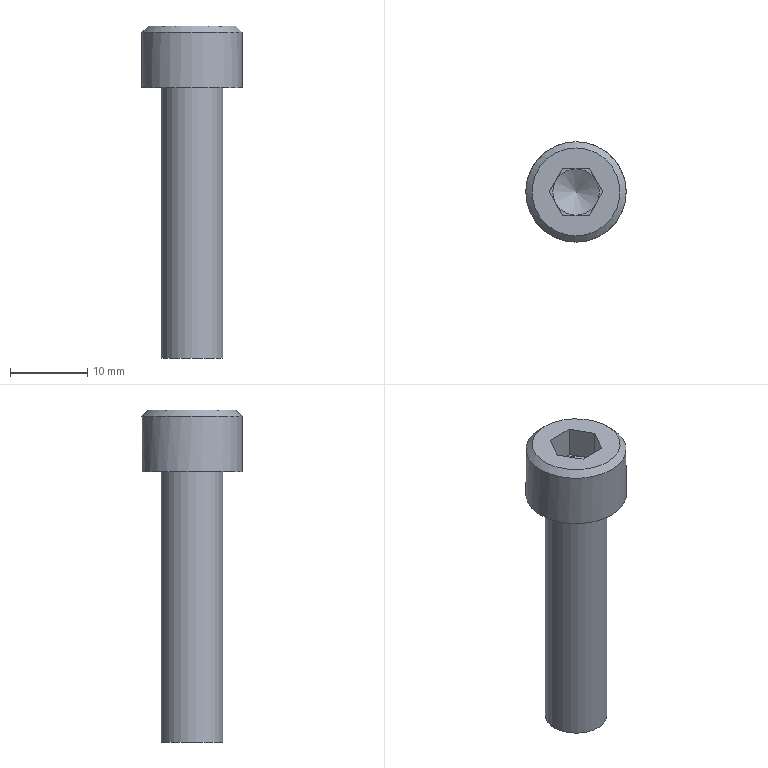Part | NX | features 5003_330_CB8-35 2 | 1 solid | 19 faces | box 13 x 13 x 43 mm | volume 2667 mm3 | plane 15 | cylinder 2 | cone 2 | commonest cylinder face diameters 8 x1 13 x1
STEP:
#1=CARTESIAN_POINT('',(-1.475,-243.8,-208.5));
#2=VERTEX_POINT('',#1);
#3=CARTESIAN_POINT('',(-1.475,-249.5,-208.5));
#4=DIRECTION('',(0.,0.,-1.));
#5=DIRECTION('',(0.,1.,0.));
#6=AXIS2_PLACEMENT_3D('',#3,#4,#5);
#7=CIRCLE('',#6,5.7);
#8=EDGE_CURVE('',#2,#2,#7,.F.);
#9=ORIENTED_EDGE('',*,*,#8,.T.);
#10=EDGE_LOOP('',(#9));
#11=FACE_BOUND('',#10,.T.);
#12=CARTESIAN_POINT('',(-4.939,-249.5,-208.5));
#13=VERTEX_POINT('',#12);
#14=CARTESIAN_POINT('',(-3.207,-252.5,-208.5));
#15=VERTEX_POINT('',#14);
#16=CARTESIAN_POINT('',(-4.939,-249.5,-208.5));
#17=DIRECTION('',(0.5,-0.866,0.));
#18=VECTOR('',#17,1000.);
#19=LINE('',#16,#18);
#20=EDGE_CURVE('',#13,#15,#19,.T.);
#21=ORIENTED_EDGE('',*,*,#20,.F.);
#22=CARTESIAN_POINT('',(-3.207,-246.5,-208.5));
#23=VERTEX_POINT('',#22);
#24=CARTESIAN_POINT('',(-3.207,-246.5,-208.5));
#25=DIRECTION('',(-0.5,-0.866,0.));
#26=VECTOR('',#25,1000.);
#27=LINE('',#24,#26);
#28=EDGE_CURVE('',#23,#13,#27,.T.);
#29=ORIENTED_EDGE('',*,*,#28,.F.);
#30=CARTESIAN_POINT('',(0.2571,-246.5,-208.5));
#31=VERTEX_POINT('',#30);
#32=CARTESIAN_POINT('',(0.2571,-246.5,-208.5));
#33=DIRECTION('',(-1.,0.,0.));
#34=VECTOR('',#33,1000.);
#35=LINE('',#32,#34);
#36=EDGE_CURVE('',#31,#23,#35,.T.);
#37=ORIENTED_EDGE('',*,*,#36,.F.);
#38=CARTESIAN_POINT('',(1.989,-249.5,-208.5));
#39=VERTEX_POINT('',#38);
#40=CARTESIAN_POINT('',(1.989,-249.5,-208.5));
#41=DIRECTION('',(-0.5,0.866,0.));
#42=VECTOR('',#41,1000.);
#43=LINE('',#40,#42);
#44=EDGE_CURVE('',#39,#31,#43,.T.);
#45=ORIENTED_EDGE('',*,*,#44,.F.);
#46=CARTESIAN_POINT('',(0.2571,-252.5,-208.5));
#47=VERTEX_POINT('',#46);
#48=CARTESIAN_POINT('',(0.2571,-252.5,-208.5));
#49=DIRECTION('',(0.5,0.866,0.));
#50=VECTOR('',#49,1000.);
#51=LINE('',#48,#50);
#52=EDGE_CURVE('',#47,#39,#51,.T.);
#53=ORIENTED_EDGE('',*,*,#52,.F.);
#54=CARTESIAN_POINT('',(-3.207,-252.5,-208.5));
#55=DIRECTION('',(1.,0.,0.));
#56=VECTOR('',#55,1000.);
#57=LINE('',#54,#56);
#58=EDGE_CURVE('',#15,#47,#57,.T.);
#59=ORIENTED_EDGE('',*,*,#58,.F.);
#60=EDGE_LOOP('',(#21,#29,#37,#45,#53,#59));
#61=FACE_BOUND('',#60,.T.);
#62=CARTESIAN_POINT('',(5.025,-249.5,-208.5));
#63=DIRECTION('',(0.,0.,-1.));
#64=DIRECTION('',(0.,1.,0.));
#65=AXIS2_PLACEMENT_3D('',#62,#63,#64);
#66=PLANE('',#65);
#67=ADVANCED_FACE('',(#11,#61),#66,.F.);
#68=CARTESIAN_POINT('',(-1.475,-253.5,-251.5));
#69=VERTEX_POINT('',#68);
#70=CARTESIAN_POINT('',(-1.475,-249.5,-251.5));
#71=DIRECTION('',(0.,0.,1.));
#72=DIRECTION('',(0.,-1.,0.));
#73=AXIS2_PLACEMENT_3D('',#70,#71,#72);
#74=CIRCLE('',#73,4.);
#75=EDGE_CURVE('',#69,#69,#74,.T.);
#76=ORIENTED_EDGE('',*,*,#75,.F.);
#77=EDGE_LOOP('',(#76));
#78=FACE_BOUND('',#77,.T.);
#79=CARTESIAN_POINT('',(-1.475,-249.5,-251.5));
#80=DIRECTION('',(0.,0.,1.));
#81=DIRECTION('',(0.,-1.,0.));
#82=AXIS2_PLACEMENT_3D('',#79,#80,#81);
#83=PLANE('',#82);
#84=ADVANCED_FACE('',(#78),#83,.F.);
#85=CARTESIAN_POINT('',(-1.475,-253.5,-216.5));
#86=VERTEX_POINT('',#85);
#87=CARTESIAN_POINT('',(-1.475,-249.5,-216.5));
#88=DIRECTION('',(0.,0.,1.));
#89=DIRECTION('',(0.,-1.,0.));
#90=AXIS2_PLACEMENT_3D('',#87,#88,#89);
#91=CIRCLE('',#90,4.);
#92=EDGE_CURVE('',#86,#86,#91,.T.);
#93=ORIENTED_EDGE('',*,*,#92,.F.);
#94=EDGE_LOOP('',(#93));
#95=FACE_BOUND('',#94,.T.);
#96=ORIENTED_EDGE('',*,*,#75,.T.);
#97=EDGE_LOOP('',(#96));
#98=FACE_BOUND('',#97,.T.);
#99=CARTESIAN_POINT('',(-1.475,-249.5,-208.5));
#100=DIRECTION('',(0.,0.,1.));
#101=DIRECTION('',(0.,-1.,0.));
#102=AXIS2_PLACEMENT_3D('',#99,#100,#101);
#103=CYLINDRICAL_SURFACE('',#102,4.);
#104=ADVANCED_FACE('',(#95,#98),#103,.T.);
#105=CARTESIAN_POINT('',(-1.475,-256.,-216.5));
#106=VERTEX_POINT('',#105);
#107=CARTESIAN_POINT('',(-1.475,-249.5,-216.5));
#108=DIRECTION('',(0.,0.,1.));
#109=DIRECTION('',(0.,-1.,0.));
#110=AXIS2_PLACEMENT_3D('',#107,#108,#109);
#111=CIRCLE('',#110,6.5);
#112=EDGE_CURVE('',#106,#106,#111,.T.);
#113=ORIENTED_EDGE('',*,*,#112,.F.);
#114=EDGE_LOOP('',(#113));
#115=FACE_BOUND('',#114,.T.);
#116=ORIENTED_EDGE('',*,*,#92,.T.);
#117=EDGE_LOOP('',(#116));
#118=FACE_BOUND('',#117,.T.);
#119=CARTESIAN_POINT('',(2.525,-249.5,-216.5));
#120=DIRECTION('',(0.,0.,1.));
#121=DIRECTION('',(0.,-1.,0.));
#122=AXIS2_PLACEMENT_3D('',#119,#120,#121);
#123=PLANE('',#122);
#124=ADVANCED_FACE('',(#115,#118),#123,.F.);
#125=CARTESIAN_POINT('',(-1.475,-243.,-209.3));
#126=VERTEX_POINT('',#125);
#127=CARTESIAN_POINT('',(-1.475,-249.5,-209.3));
#128=DIRECTION('',(0.,0.,-1.));
#129=DIRECTION('',(0.,1.,0.));
#130=AXIS2_PLACEMENT_3D('',#127,#128,#129);
#131=CIRCLE('',#130,6.5);
#132=EDGE_CURVE('',#126,#126,#131,.T.);
#133=ORIENTED_EDGE('',*,*,#132,.T.);
#134=EDGE_LOOP('',(#133));
#135=FACE_BOUND('',#134,.T.);
#136=ORIENTED_EDGE('',*,*,#112,.T.);
#137=EDGE_LOOP('',(#136));
#138=FACE_BOUND('',#137,.T.);
#139=CARTESIAN_POINT('',(-1.475,-249.5,-208.5));
#140=DIRECTION('',(0.,0.,1.));
#141=DIRECTION('',(0.,-1.,0.));
#142=AXIS2_PLACEMENT_3D('',#139,#140,#141);
#143=CYLINDRICAL_SURFACE('',#142,6.5);
#144=ADVANCED_FACE('',(#135,#138),#143,.T.);
#145=ORIENTED_EDGE('',*,*,#132,.F.);
#146=EDGE_LOOP('',(#145));
#147=FACE_BOUND('',#146,.T.);
#148=ORIENTED_EDGE('',*,*,#8,.F.);
#149=EDGE_LOOP('',(#148));
#150=FACE_BOUND('',#149,.T.);
#151=CARTESIAN_POINT('',(-1.475,-249.5,-208.5));
#152=DIRECTION('',(0.,0.,-1.));
#153=DIRECTION('',(0.,1.,0.));
#154=AXIS2_PLACEMENT_3D('',#151,#152,#153);
#155=CONICAL_SURFACE('',#154,5.7,0.7854);
#156=ADVANCED_FACE('',(#147,#150),#155,.T.);
#157=CARTESIAN_POINT('',(-3.207,-246.5,-212.5));
#158=VERTEX_POINT('',#157);
#159=CARTESIAN_POINT('',(-4.073,-248.,-212.5));
#160=VERTEX_POINT('',#159);
#161=CARTESIAN_POINT('',(-3.207,-246.5,-212.5));
#162=DIRECTION('',(-0.5,-0.866,0.));
#163=VECTOR('',#162,1000.);
#164=LINE('',#161,#163);
#165=EDGE_CURVE('',#158,#160,#164,.T.);
#166=ORIENTED_EDGE('',*,*,#165,.F.);
#167=CARTESIAN_POINT('',(-3.207,-246.5,-212.5));
#168=DIRECTION('',(0.,0.,1.));
#169=VECTOR('',#168,1000.);
#170=LINE('',#167,#169);
#171=EDGE_CURVE('',#158,#23,#170,.T.);
#172=ORIENTED_EDGE('',*,*,#171,.T.);
#173=ORIENTED_EDGE('',*,*,#28,.T.);
#174=CARTESIAN_POINT('',(-4.939,-249.5,-212.5));
#175=VERTEX_POINT('',#174);
#176=CARTESIAN_POINT('',(-4.939,-249.5,-212.5));
#177=DIRECTION('',(0.,0.,1.));
#178=VECTOR('',#177,1000.);
#179=LINE('',#176,#178);
#180=EDGE_CURVE('',#175,#13,#179,.T.);
#181=ORIENTED_EDGE('',*,*,#180,.F.);
#182=CARTESIAN_POINT('',(-3.207,-246.5,-212.5));
#183=DIRECTION('',(-0.5,-0.866,0.));
#184=VECTOR('',#183,1000.);
#185=LINE('',#182,#184);
#186=EDGE_CURVE('',#160,#175,#185,.T.);
#187=ORIENTED_EDGE('',*,*,#186,.F.);
#188=EDGE_LOOP('',(#166,#172,#173,#181,#187));
#189=FACE_BOUND('',#188,.T.);
#190=CARTESIAN_POINT('',(-3.207,-246.5,-212.5));
#191=DIRECTION('',(-0.866,0.5,0.));
#192=DIRECTION('',(0.5,0.866,0.));
#193=AXIS2_PLACEMENT_3D('',#190,#191,#192);
#194=PLANE('',#193);
#195=ADVANCED_FACE('',(#189),#194,.F.);
#196=CARTESIAN_POINT('',(0.2571,-246.5,-212.5));
#197=VERTEX_POINT('',#196);
#198=CARTESIAN_POINT('',(-1.475,-246.5,-212.5));
#199=VERTEX_POINT('',#198);
#200=CARTESIAN_POINT('',(0.2571,-246.5,-212.5));
#201=DIRECTION('',(-1.,0.,0.));
#202=VECTOR('',#201,1000.);
#203=LINE('',#200,#202);
#204=EDGE_CURVE('',#197,#199,#203,.T.);
#205=ORIENTED_EDGE('',*,*,#204,.F.);
#206=CARTESIAN_POINT('',(0.2571,-246.5,-212.5));
#207=DIRECTION('',(0.,0.,1.));
#208=VECTOR('',#207,1000.);
#209=LINE('',#206,#208);
#210=EDGE_CURVE('',#197,#31,#209,.T.);
#211=ORIENTED_EDGE('',*,*,#210,.T.);
#212=ORIENTED_EDGE('',*,*,#36,.T.);
#213=ORIENTED_EDGE('',*,*,#171,.F.);
#214=CARTESIAN_POINT('',(0.2571,-246.5,-212.5));
#215=DIRECTION('',(-1.,0.,0.));
#216=VECTOR('',#215,1000.);
#217=LINE('',#214,#216);
#218=EDGE_CURVE('',#199,#158,#217,.T.);
#219=ORIENTED_EDGE('',*,*,#218,.F.);
#220=EDGE_LOOP('',(#205,#211,#212,#213,#219));
#221=FACE_BOUND('',#220,.T.);
#222=CARTESIAN_POINT('',(0.2571,-246.5,-212.5));
#223=DIRECTION('',(0.,1.,0.));
#224=DIRECTION('',(0.,0.,1.));
#225=AXIS2_PLACEMENT_3D('',#222,#223,#224);
#226=PLANE('',#225);
#227=ADVANCED_FACE('',(#221),#226,.F.);
#228=CARTESIAN_POINT('',(1.989,-249.5,-212.5));
#229=VERTEX_POINT('',#228);
#230=CARTESIAN_POINT('',(1.123,-248.,-212.5));
#231=VERTEX_POINT('',#230);
#232=CARTESIAN_POINT('',(1.989,-249.5,-212.5));
#233=DIRECTION('',(-0.5,0.866,0.));
#234=VECTOR('',#233,1000.);
#235=LINE('',#232,#234);
#236=EDGE_CURVE('',#229,#231,#235,.T.);
#237=ORIENTED_EDGE('',*,*,#236,.F.);
#238=CARTESIAN_POINT('',(1.989,-249.5,-212.5));
#239=DIRECTION('',(0.,0.,1.));
#240=VECTOR('',#239,1000.);
#241=LINE('',#238,#240);
#242=EDGE_CURVE('',#229,#39,#241,.T.);
#243=ORIENTED_EDGE('',*,*,#242,.T.);
#244=ORIENTED_EDGE('',*,*,#44,.T.);
#245=ORIENTED_EDGE('',*,*,#210,.F.);
#246=CARTESIAN_POINT('',(1.989,-249.5,-212.5));
#247=DIRECTION('',(-0.5,0.866,0.));
#248=VECTOR('',#247,1000.);
#249=LINE('',#246,#248);
#250=EDGE_CURVE('',#231,#197,#249,.T.);
#251=ORIENTED_EDGE('',*,*,#250,.F.);
#252=EDGE_LOOP('',(#237,#243,#244,#245,#251));
#253=FACE_BOUND('',#252,.T.);
#254=CARTESIAN_POINT('',(1.989,-249.5,-212.5));
#255=DIRECTION('',(0.866,0.5,0.));
#256=DIRECTION('',(0.5,-0.866,0.));
#257=AXIS2_PLACEMENT_3D('',#254,#255,#256);
#258=PLANE('',#257);
#259=ADVANCED_FACE('',(#253),#258,.F.);
#260=CARTESIAN_POINT('',(0.2571,-252.5,-212.5));
#261=VERTEX_POINT('',#260);
#262=CARTESIAN_POINT('',(1.123,-251.,-212.5));
#263=VERTEX_POINT('',#262);
#264=CARTESIAN_POINT('',(0.2571,-252.5,-212.5));
#265=DIRECTION('',(0.5,0.866,0.));
#266=VECTOR('',#265,1000.);
#267=LINE('',#264,#266);
#268=EDGE_CURVE('',#261,#263,#267,.T.);
#269=ORIENTED_EDGE('',*,*,#268,.F.);
#270=CARTESIAN_POINT('',(0.2571,-252.5,-212.5));
#271=DIRECTION('',(0.,0.,1.));
#272=VECTOR('',#271,1000.);
#273=LINE('',#270,#272);
#274=EDGE_CURVE('',#261,#47,#273,.T.);
#275=ORIENTED_EDGE('',*,*,#274,.T.);
#276=ORIENTED_EDGE('',*,*,#52,.T.);
#277=ORIENTED_EDGE('',*,*,#242,.F.);
#278=CARTESIAN_POINT('',(0.2571,-252.5,-212.5));
#279=DIRECTION('',(0.5,0.866,0.));
#280=VECTOR('',#279,1000.);
#281=LINE('',#278,#280);
#282=EDGE_CURVE('',#263,#229,#281,.T.);
#283=ORIENTED_EDGE('',*,*,#282,.F.);
#284=EDGE_LOOP('',(#269,#275,#276,#277,#283));
#285=FACE_BOUND('',#284,.T.);
#286=CARTESIAN_POINT('',(0.2571,-252.5,-212.5));
#287=DIRECTION('',(0.866,-0.5,0.));
#288=DIRECTION('',(-0.5,-0.866,0.));
#289=AXIS2_PLACEMENT_3D('',#286,#287,#288);
#290=PLANE('',#289);
#291=ADVANCED_FACE('',(#285),#290,.F.);
#292=CARTESIAN_POINT('',(-3.207,-252.5,-212.5));
#293=VERTEX_POINT('',#292);
#294=CARTESIAN_POINT('',(-1.475,-252.5,-212.5));
#295=VERTEX_POINT('',#294);
#296=CARTESIAN_POINT('',(-3.207,-252.5,-212.5));
#297=DIRECTION('',(1.,0.,0.));
#298=VECTOR('',#297,1000.);
#299=LINE('',#296,#298);
#300=EDGE_CURVE('',#293,#295,#299,.T.);
#301=ORIENTED_EDGE('',*,*,#300,.F.);
#302=CARTESIAN_POINT('',(-3.207,-252.5,-212.5));
#303=DIRECTION('',(0.,0.,1.));
#304=VECTOR('',#303,1000.);
#305=LINE('',#302,#304);
#306=EDGE_CURVE('',#293,#15,#305,.T.);
#307=ORIENTED_EDGE('',*,*,#306,.T.);
#308=ORIENTED_EDGE('',*,*,#58,.T.);
#309=ORIENTED_EDGE('',*,*,#274,.F.);
#310=CARTESIAN_POINT('',(-3.207,-252.5,-212.5));
#311=DIRECTION('',(1.,0.,0.));
#312=VECTOR('',#311,1000.);
#313=LINE('',#310,#312);
#314=EDGE_CURVE('',#295,#261,#313,.T.);
#315=ORIENTED_EDGE('',*,*,#314,.F.);
#316=EDGE_LOOP('',(#301,#307,#308,#309,#315));
#317=FACE_BOUND('',#316,.T.);
#318=CARTESIAN_POINT('',(-3.207,-252.5,-212.5));
#319=DIRECTION('',(0.,-1.,0.));
#320=DIRECTION('',(-1.,0.,0.));
#321=AXIS2_PLACEMENT_3D('',#318,#319,#320);
#322=PLANE('',#321);
#323=ADVANCED_FACE('',(#317),#322,.F.);
#324=CARTESIAN_POINT('',(-4.073,-251.,-212.5));
#325=VERTEX_POINT('',#324);
#326=CARTESIAN_POINT('',(-4.939,-249.5,-212.5));
#327=DIRECTION('',(0.5,-0.866,0.));
#328=VECTOR('',#327,1000.);
#329=LINE('',#326,#328);
#330=EDGE_CURVE('',#175,#325,#329,.T.);
#331=ORIENTED_EDGE('',*,*,#330,.F.);
#332=ORIENTED_EDGE('',*,*,#180,.T.);
#333=ORIENTED_EDGE('',*,*,#20,.T.);
#334=ORIENTED_EDGE('',*,*,#306,.F.);
#335=CARTESIAN_POINT('',(-4.939,-249.5,-212.5));
#336=DIRECTION('',(0.5,-0.866,0.));
#337=VECTOR('',#336,1000.);
#338=LINE('',#335,#337);
#339=EDGE_CURVE('',#325,#293,#338,.T.);
#340=ORIENTED_EDGE('',*,*,#339,.F.);
#341=EDGE_LOOP('',(#331,#332,#333,#334,#340));
#342=FACE_BOUND('',#341,.T.);
#343=CARTESIAN_POINT('',(-4.939,-249.5,-212.5));
#344=DIRECTION('',(-0.866,-0.5,0.));
#345=DIRECTION('',(-0.5,0.866,0.));
#346=AXIS2_PLACEMENT_3D('',#343,#344,#345);
#347=PLANE('',#346);
#348=ADVANCED_FACE('',(#342),#347,.F.);
#349=ORIENTED_EDGE('',*,*,#314,.T.);
#350=ORIENTED_EDGE('',*,*,#268,.T.);
#351=CARTESIAN_POINT('',(-1.475,-249.5,-212.5));
#352=DIRECTION('',(0.,0.,1.));
#353=DIRECTION('',(-1.,0.,0.));
#354=AXIS2_PLACEMENT_3D('',#351,#352,#353);
#355=CIRCLE('',#354,3.);
#356=EDGE_CURVE('',#295,#263,#355,.T.);
#357=ORIENTED_EDGE('',*,*,#356,.F.);
#358=EDGE_LOOP('',(#349,#350,#357));
#359=FACE_BOUND('',#358,.T.);
#360=CARTESIAN_POINT('',(-1.475,-249.5,-212.5));
#361=DIRECTION('',(0.,0.,1.));
#362=DIRECTION('',(0.,-1.,0.));
#363=AXIS2_PLACEMENT_3D('',#360,#361,#362);
#364=PLANE('',#363);
#365=ADVANCED_FACE('',(#359),#364,.T.);
#366=ORIENTED_EDGE('',*,*,#282,.T.);
#367=ORIENTED_EDGE('',*,*,#236,.T.);
#368=CARTESIAN_POINT('',(-1.475,-249.5,-212.5));
#369=DIRECTION('',(0.,0.,1.));
#370=DIRECTION('',(-1.,0.,0.));
#371=AXIS2_PLACEMENT_3D('',#368,#369,#370);
#372=CIRCLE('',#371,3.);
#373=EDGE_CURVE('',#263,#231,#372,.T.);
#374=ORIENTED_EDGE('',*,*,#373,.F.);
#375=EDGE_LOOP('',(#366,#367,#374));
#376=FACE_BOUND('',#375,.T.);
#377=CARTESIAN_POINT('',(-1.475,-249.5,-212.5));
#378=DIRECTION('',(0.,0.,1.));
#379=DIRECTION('',(0.,-1.,0.));
#380=AXIS2_PLACEMENT_3D('',#377,#378,#379);
#381=PLANE('',#380);
#382=ADVANCED_FACE('',(#376),#381,.T.);
#383=ORIENTED_EDGE('',*,*,#250,.T.);
#384=ORIENTED_EDGE('',*,*,#204,.T.);
#385=CARTESIAN_POINT('',(-1.475,-249.5,-212.5));
#386=DIRECTION('',(0.,0.,1.));
#387=DIRECTION('',(-1.,0.,0.));
#388=AXIS2_PLACEMENT_3D('',#385,#386,#387);
#389=CIRCLE('',#388,3.);
#390=EDGE_CURVE('',#231,#199,#389,.T.);
#391=ORIENTED_EDGE('',*,*,#390,.F.);
#392=EDGE_LOOP('',(#383,#384,#391));
#393=FACE_BOUND('',#392,.T.);
#394=CARTESIAN_POINT('',(-1.475,-249.5,-212.5));
#395=DIRECTION('',(0.,0.,1.));
#396=DIRECTION('',(0.,-1.,0.));
#397=AXIS2_PLACEMENT_3D('',#394,#395,#396);
#398=PLANE('',#397);
#399=ADVANCED_FACE('',(#393),#398,.T.);
#400=ORIENTED_EDGE('',*,*,#218,.T.);
#401=ORIENTED_EDGE('',*,*,#165,.T.);
#402=CARTESIAN_POINT('',(-1.475,-249.5,-212.5));
#403=DIRECTION('',(0.,0.,1.));
#404=DIRECTION('',(-1.,0.,0.));
#405=AXIS2_PLACEMENT_3D('',#402,#403,#404);
#406=CIRCLE('',#405,3.);
#407=EDGE_CURVE('',#199,#160,#406,.T.);
#408=ORIENTED_EDGE('',*,*,#407,.F.);
#409=EDGE_LOOP('',(#400,#401,#408));
#410=FACE_BOUND('',#409,.T.);
#411=CARTESIAN_POINT('',(-1.475,-249.5,-212.5));
#412=DIRECTION('',(0.,0.,1.));
#413=DIRECTION('',(0.,-1.,0.));
#414=AXIS2_PLACEMENT_3D('',#411,#412,#413);
#415=PLANE('',#414);
#416=ADVANCED_FACE('',(#410),#415,.T.);
#417=ORIENTED_EDGE('',*,*,#186,.T.);
#418=ORIENTED_EDGE('',*,*,#330,.T.);
#419=CARTESIAN_POINT('',(-1.475,-249.5,-212.5));
#420=DIRECTION('',(0.,0.,1.));
#421=DIRECTION('',(-1.,0.,0.));
#422=AXIS2_PLACEMENT_3D('',#419,#420,#421);
#423=CIRCLE('',#422,3.);
#424=EDGE_CURVE('',#160,#325,#423,.T.);
#425=ORIENTED_EDGE('',*,*,#424,.F.);
#426=EDGE_LOOP('',(#417,#418,#425));
#427=FACE_BOUND('',#426,.T.);
#428=CARTESIAN_POINT('',(-1.475,-249.5,-212.5));
#429=DIRECTION('',(0.,0.,1.));
#430=DIRECTION('',(0.,-1.,0.));
#431=AXIS2_PLACEMENT_3D('',#428,#429,#430);
#432=PLANE('',#431);
#433=ADVANCED_FACE('',(#427),#432,.T.);
#434=ORIENTED_EDGE('',*,*,#339,.T.);
#435=ORIENTED_EDGE('',*,*,#300,.T.);
#436=CARTESIAN_POINT('',(-1.475,-249.5,-212.5));
#437=DIRECTION('',(0.,0.,1.));
#438=DIRECTION('',(-1.,0.,0.));
#439=AXIS2_PLACEMENT_3D('',#436,#437,#438);
#440=CIRCLE('',#439,3.);
#441=EDGE_CURVE('',#325,#295,#440,.T.);
#442=ORIENTED_EDGE('',*,*,#441,.F.);
#443=EDGE_LOOP('',(#434,#435,#442));
#444=FACE_BOUND('',#443,.T.);
#445=CARTESIAN_POINT('',(-1.475,-249.5,-212.5));
#446=DIRECTION('',(0.,0.,1.));
#447=DIRECTION('',(0.,-1.,0.));
#448=AXIS2_PLACEMENT_3D('',#445,#446,#447);
#449=PLANE('',#448);
#450=ADVANCED_FACE('',(#444),#449,.T.);
#451=ORIENTED_EDGE('',*,*,#441,.T.);
#452=ORIENTED_EDGE('',*,*,#356,.T.);
#453=ORIENTED_EDGE('',*,*,#373,.T.);
#454=ORIENTED_EDGE('',*,*,#390,.T.);
#455=ORIENTED_EDGE('',*,*,#407,.T.);
#456=ORIENTED_EDGE('',*,*,#424,.T.);
#457=EDGE_LOOP('',(#451,#452,#453,#454,#455,#456));
#458=FACE_BOUND('',#457,.T.);
#459=CARTESIAN_POINT('',(-1.475,-249.5,-214.303));
#460=VERTEX_POINT('',#459);
#461=VERTEX_LOOP('',#460);
#462=FACE_BOUND('',#461,.T.);
#463=CARTESIAN_POINT('',(-1.475,-249.5,-214.303));
#464=DIRECTION('',(0.,0.,1.));
#465=DIRECTION('',(-1.,0.,0.));
#466=AXIS2_PLACEMENT_3D('',#463,#464,#465);
#467=CONICAL_SURFACE('',#466,0.,1.03);
#468=ADVANCED_FACE('',(#458,#462),#467,.F.);
#469=CLOSED_SHELL('',(#67,#84,#104,#124,#144,#156,#195,#227,#259,#291,#323,#348,#365,#382,#399,#416,#433,#450,#468));
#470=MANIFOLD_SOLID_BREP('',#469);
#471=(LENGTH_UNIT()NAMED_UNIT(*)SI_UNIT(.MILLI.,.METRE.));
#472=UNCERTAINTY_MEASURE_WITH_UNIT(LENGTH_MEASURE(0.00001),#471,'','');
#473=(NAMED_UNIT(*)PLANE_ANGLE_UNIT()SI_UNIT($,.RADIAN.));
#474=(NAMED_UNIT(*)SI_UNIT($,.STERADIAN.)SOLID_ANGLE_UNIT());
#475=(GEOMETRIC_REPRESENTATION_CONTEXT(3)GLOBAL_UNCERTAINTY_ASSIGNED_CONTEXT((#472))GLOBAL_UNIT_ASSIGNED_CONTEXT((#471,#473,#474))REPRESENTATION_CONTEXT('',''));
#476=ADVANCED_BREP_SHAPE_REPRESENTATION('',(#470),#475);